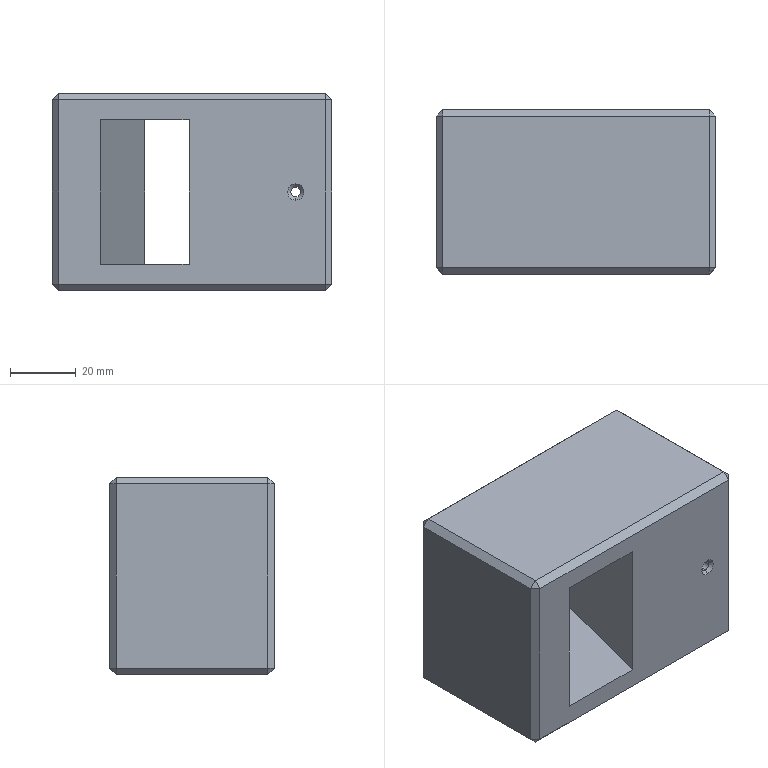Part | STEP file | Gaveta - Torre - 4 cav | 1 solid | 47 faces | box 85 x 50 x 60 mm | volume 180516 mm3 | plane 31 | cone 8 | cylinder 8 | commonest cylinder face diameters 6 x4 3 x2 27 x2